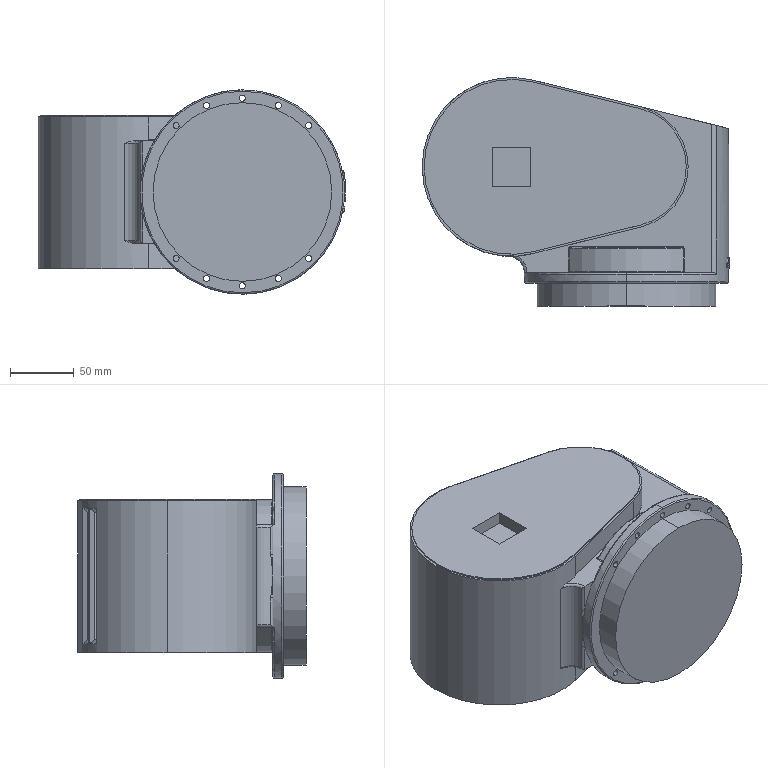Part | SolidWorks | features ICE 11, CirPattern 3, Fillet 3, MirrorPattern 2, 3DProfileFeature 1, Chamfer 1, Emboss 1, Extrusion 1, HoleWzd 1 | 1 solid | 242 faces | box 241 x 179 x 160 mm | volume 3546653 mm3 | cylinder 73 | plane 72 | spline 60 | torus 33 | cone 4 | commonest cylinder face diameters 4.8 x20 9 x20 2 x6 162 x5 140 x4 93.826 x3